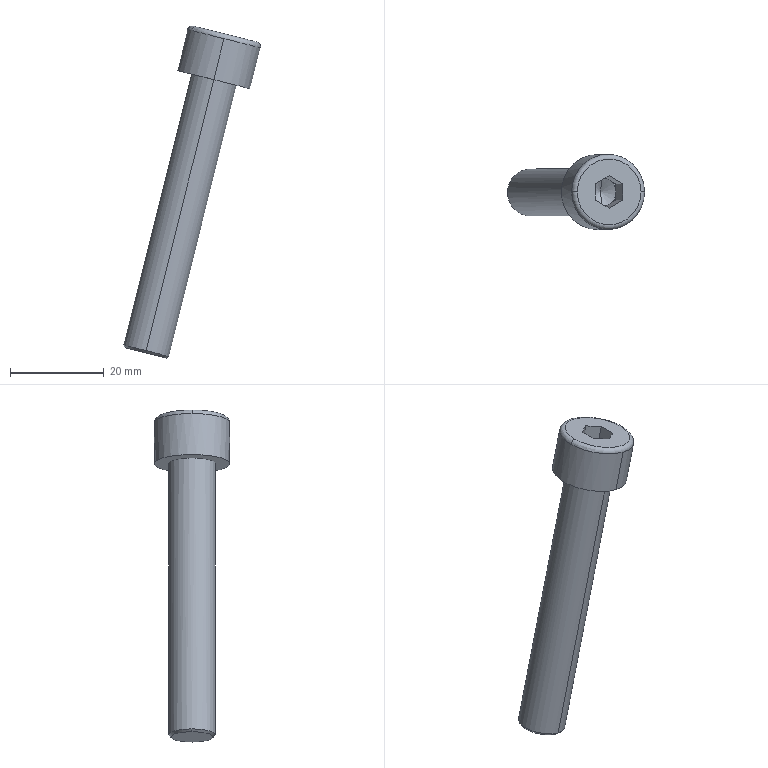Part | SolidWorks | features BaseBody 1 | 1 solid | 25 faces | box 29.213 x 16 x 70.733 mm | volume 6505 mm3 | plane 15 | cone 4 | cylinder 4 | torus 2 | commonest cylinder face diameters 10 x2 16 x2
STEP:
#1=CARTESIAN_POINT('',(-428.449,-4.,429.111));
#2=VERTEX_POINT('',#1);
#3=CARTESIAN_POINT('',(-414.865,-4.,425.724));
#4=VERTEX_POINT('',#3);
#5=CARTESIAN_POINT('',(-421.657,-4.,427.418));
#6=DIRECTION('',(0.2419,0.,0.9703));
#7=DIRECTION('',(-0.9703,0.,0.2419));
#8=AXIS2_PLACEMENT_3D('',#5,#6,#7);
#9=CIRCLE('',#8,7.);
#10=EDGE_CURVE('',#2,#4,#9,.T.);
#11=ORIENTED_EDGE('',*,*,#10,.F.);
#12=CARTESIAN_POINT('',(-429.661,-4.,428.382));
#13=VERTEX_POINT('',#12);
#14=CARTESIAN_POINT('',(-428.691,-4.,428.14));
#15=DIRECTION('',(0.,-1.,0.));
#16=DIRECTION('',(1.,0.,0.));
#17=AXIS2_PLACEMENT_3D('',#14,#15,#16);
#18=CIRCLE('',#17,1.);
#19=EDGE_CURVE('',#2,#13,#18,.T.);
#20=ORIENTED_EDGE('',*,*,#19,.T.);
#21=CARTESIAN_POINT('',(-421.899,-12.,426.447));
#22=VERTEX_POINT('',#21);
#23=CARTESIAN_POINT('',(-421.899,-4.,426.447));
#24=DIRECTION('',(-0.2419,0.,-0.9703));
#25=DIRECTION('',(-0.9703,0.,0.2419));
#26=AXIS2_PLACEMENT_3D('',#23,#24,#25);
#27=CIRCLE('',#26,8.);
#28=EDGE_CURVE('',#22,#13,#27,.T.);
#29=ORIENTED_EDGE('',*,*,#28,.F.);
#30=CARTESIAN_POINT('',(-414.136,-4.,424.512));
#31=VERTEX_POINT('',#30);
#32=CARTESIAN_POINT('',(-421.899,-4.,426.447));
#33=DIRECTION('',(-0.2419,0.,-0.9703));
#34=DIRECTION('',(-0.9703,0.,0.2419));
#35=AXIS2_PLACEMENT_3D('',#32,#33,#34);
#36=CIRCLE('',#35,8.);
#37=EDGE_CURVE('',#31,#22,#36,.T.);
#38=ORIENTED_EDGE('',*,*,#37,.F.);
#39=CARTESIAN_POINT('',(-415.107,-4.,424.754));
#40=DIRECTION('',(0.,1.,0.));
#41=DIRECTION('',(0.,0.,1.));
#42=AXIS2_PLACEMENT_3D('',#39,#40,#41);
#43=CIRCLE('',#42,1.);
#44=EDGE_CURVE('',#4,#31,#43,.T.);
#45=ORIENTED_EDGE('',*,*,#44,.F.);
#46=EDGE_LOOP('',(#11,#20,#29,#38,#45));
#47=FACE_OUTER_BOUND('',#46,.T.);
#48=CARTESIAN_POINT('',(-421.899,-4.,426.447));
#49=DIRECTION('',(-0.2419,0.,-0.9703));
#50=DIRECTION('',(0.9703,0.,-0.2419));
#51=AXIS2_PLACEMENT_3D('',#48,#49,#50);
#52=TOROIDAL_SURFACE('',#51,7.,1.);
#53=ADVANCED_FACE('',(#47),#52,.T.);
#54=CARTESIAN_POINT('',(-434.222,-4.,358.408));
#55=VERTEX_POINT('',#54);
#56=CARTESIAN_POINT('',(-442.955,-4.,360.585));
#57=VERTEX_POINT('',#56);
#58=CARTESIAN_POINT('',(-438.589,-4.,359.496));
#59=DIRECTION('',(-0.2419,0.,-0.9703));
#60=DIRECTION('',(-0.9703,0.,0.2419));
#61=AXIS2_PLACEMENT_3D('',#58,#59,#60);
#62=CIRCLE('',#61,4.5);
#63=EDGE_CURVE('',#55,#57,#62,.T.);
#64=ORIENTED_EDGE('',*,*,#63,.F.);
#65=CARTESIAN_POINT('',(-433.616,-4.,358.772));
#66=VERTEX_POINT('',#65);
#67=CARTESIAN_POINT('',(-434.222,-4.,358.408));
#68=DIRECTION('',(0.8571,0.,0.5151));
#69=VECTOR('',#68,1000.);
#70=LINE('',#67,#69);
#71=EDGE_CURVE('',#55,#66,#70,.T.);
#72=ORIENTED_EDGE('',*,*,#71,.T.);
#73=CARTESIAN_POINT('',(-438.468,-9.,359.981));
#74=VERTEX_POINT('',#73);
#75=CARTESIAN_POINT('',(-438.468,-4.,359.981));
#76=DIRECTION('',(0.2419,0.,0.9703));
#77=DIRECTION('',(0.9703,0.,-0.2419));
#78=AXIS2_PLACEMENT_3D('',#75,#76,#77);
#79=CIRCLE('',#78,5.);
#80=EDGE_CURVE('',#74,#66,#79,.T.);
#81=ORIENTED_EDGE('',*,*,#80,.F.);
#82=CARTESIAN_POINT('',(-443.319,-4.,361.191));
#83=VERTEX_POINT('',#82);
#84=CARTESIAN_POINT('',(-438.468,-4.,359.981));
#85=DIRECTION('',(0.2419,0.,0.9703));
#86=DIRECTION('',(0.9703,0.,-0.2419));
#87=AXIS2_PLACEMENT_3D('',#84,#85,#86);
#88=CIRCLE('',#87,5.);
#89=EDGE_CURVE('',#83,#74,#88,.T.);
#90=ORIENTED_EDGE('',*,*,#89,.F.);
#91=CARTESIAN_POINT('',(-442.955,-4.,360.585));
#92=DIRECTION('',(-0.5151,0.,0.8571));
#93=VECTOR('',#92,1000.);
#94=LINE('',#91,#93);
#95=EDGE_CURVE('',#57,#83,#94,.T.);
#96=ORIENTED_EDGE('',*,*,#95,.F.);
#97=EDGE_LOOP('',(#64,#72,#81,#90,#96));
#98=FACE_OUTER_BOUND('',#97,.T.);
#99=CARTESIAN_POINT('',(-438.589,-4.,359.496));
#100=DIRECTION('',(0.2419,0.,0.9703));
#101=DIRECTION('',(-0.9703,0.,0.2419));
#102=AXIS2_PLACEMENT_3D('',#99,#100,#101);
#103=CONICAL_SURFACE('',#102,4.5,0.7854);
#104=ADVANCED_FACE('',(#98),#103,.T.);
#105=CARTESIAN_POINT('',(-423.527,-4.,419.915));
#106=VERTEX_POINT('',#105);
#107=CARTESIAN_POINT('',(-423.108,-1.,421.596));
#108=VERTEX_POINT('',#107);
#109=CARTESIAN_POINT('',(-423.311,-2.451,420.783));
#110=DIRECTION('',(0.1209,0.866,0.4852));
#111=VECTOR('',#110,1000.);
#112=LINE('',#109,#111);
#113=EDGE_CURVE('',#106,#108,#112,.T.);
#114=ORIENTED_EDGE('',*,*,#113,.F.);
#115=CARTESIAN_POINT('',(-423.108,-7.,421.596));
#116=VERTEX_POINT('',#115);
#117=CARTESIAN_POINT('',(-423.311,-5.549,420.783));
#118=DIRECTION('',(0.1209,-0.866,0.4852));
#119=VECTOR('',#118,1000.);
#120=LINE('',#117,#119);
#121=EDGE_CURVE('',#106,#116,#120,.T.);
#122=ORIENTED_EDGE('',*,*,#121,.T.);
#123=CARTESIAN_POINT('',(-421.653,-6.598,421.233));
#124=VERTEX_POINT('',#123);
#125=CARTESIAN_POINT('',(-423.108,-4.,421.596));
#126=DIRECTION('',(-0.2419,0.,-0.9703));
#127=DIRECTION('',(0.,-1.,0.));
#128=AXIS2_PLACEMENT_3D('',#125,#126,#127);
#129=CIRCLE('',#128,3.);
#130=EDGE_CURVE('',#124,#116,#129,.T.);
#131=ORIENTED_EDGE('',*,*,#130,.F.);
#132=CARTESIAN_POINT('',(-420.197,-4.,420.87));
#133=VERTEX_POINT('',#132);
#134=CARTESIAN_POINT('',(-423.108,-4.,421.596));
#135=DIRECTION('',(-0.2419,0.,-0.9703));
#136=DIRECTION('',(0.9703,0.,-0.2419));
#137=AXIS2_PLACEMENT_3D('',#134,#135,#136);
#138=CIRCLE('',#137,3.);
#139=EDGE_CURVE('',#133,#124,#138,.T.);
#140=ORIENTED_EDGE('',*,*,#139,.F.);
#141=CARTESIAN_POINT('',(-421.653,-1.402,421.233));
#142=VERTEX_POINT('',#141);
#143=CARTESIAN_POINT('',(-423.108,-4.,421.596));
#144=DIRECTION('',(-0.2419,0.,-0.9703));
#145=DIRECTION('',(0.4852,0.866,-0.1209));
#146=AXIS2_PLACEMENT_3D('',#143,#144,#145);
#147=CIRCLE('',#146,3.);
#148=EDGE_CURVE('',#142,#133,#147,.T.);
#149=ORIENTED_EDGE('',*,*,#148,.F.);
#150=CARTESIAN_POINT('',(-423.108,-4.,421.596));
#151=DIRECTION('',(-0.2419,0.,-0.9703));
#152=DIRECTION('',(-0.4852,0.866,0.1209));
#153=AXIS2_PLACEMENT_3D('',#150,#151,#152);
#154=CIRCLE('',#153,3.);
#155=EDGE_CURVE('',#108,#142,#154,.T.);
#156=ORIENTED_EDGE('',*,*,#155,.F.);
#157=EDGE_LOOP('',(#114,#122,#131,#140,#149,#156));
#158=FACE_OUTER_BOUND('',#157,.T.);
#159=CARTESIAN_POINT('',(-423.311,-4.,420.783));
#160=DIRECTION('',(0.2419,0.,0.9703));
#161=DIRECTION('',(0.,1.,0.));
#162=AXIS2_PLACEMENT_3D('',#159,#160,#161);
#163=CONICAL_SURFACE('',#162,1.549,1.047);
#164=ADVANCED_FACE('',(#158),#163,.F.);
#165=CARTESIAN_POINT('',(-424.076,-12.,417.715));
#166=VERTEX_POINT('',#165);
#167=CARTESIAN_POINT('',(-424.076,4.,417.715));
#168=VERTEX_POINT('',#167);
#169=CARTESIAN_POINT('',(-424.076,-4.,417.715));
#170=DIRECTION('',(-0.2419,0.,-0.9703));
#171=DIRECTION('',(-0.9703,0.,0.2419));
#172=AXIS2_PLACEMENT_3D('',#169,#170,#171);
#173=CIRCLE('',#172,8.);
#174=EDGE_CURVE('',#166,#168,#173,.T.);
#175=ORIENTED_EDGE('',*,*,#174,.F.);
#176=CARTESIAN_POINT('',(-424.076,-12.,417.715));
#177=DIRECTION('',(0.2419,0.,0.9703));
#178=VECTOR('',#177,1000.);
#179=LINE('',#176,#178);
#180=EDGE_CURVE('',#166,#22,#179,.T.);
#181=ORIENTED_EDGE('',*,*,#180,.T.);
#182=ORIENTED_EDGE('',*,*,#28,.T.);
#183=CARTESIAN_POINT('',(-421.899,4.,426.447));
#184=VERTEX_POINT('',#183);
#185=CARTESIAN_POINT('',(-421.899,-4.,426.447));
#186=DIRECTION('',(-0.2419,0.,-0.9703));
#187=DIRECTION('',(-0.9703,0.,0.2419));
#188=AXIS2_PLACEMENT_3D('',#185,#186,#187);
#189=CIRCLE('',#188,8.);
#190=EDGE_CURVE('',#13,#184,#189,.T.);
#191=ORIENTED_EDGE('',*,*,#190,.T.);
#192=CARTESIAN_POINT('',(-424.076,4.,417.715));
#193=DIRECTION('',(0.2419,0.,0.9703));
#194=VECTOR('',#193,1000.);
#195=LINE('',#192,#194);
#196=EDGE_CURVE('',#168,#184,#195,.T.);
#197=ORIENTED_EDGE('',*,*,#196,.F.);
#198=EDGE_LOOP('',(#175,#181,#182,#191,#197));
#199=FACE_OUTER_BOUND('',#198,.T.);
#200=CARTESIAN_POINT('',(-424.076,-4.,417.715));
#201=DIRECTION('',(0.2419,0.,0.9703));
#202=DIRECTION('',(0.,1.,0.));
#203=AXIS2_PLACEMENT_3D('',#200,#201,#202);
#204=CYLINDRICAL_SURFACE('',#203,8.);
#205=ADVANCED_FACE('',(#199),#204,.T.);
#206=CARTESIAN_POINT('',(-438.468,1.,359.981));
#207=VERTEX_POINT('',#206);
#208=CARTESIAN_POINT('',(-438.468,-4.,359.981));
#209=DIRECTION('',(0.2419,0.,0.9703));
#210=DIRECTION('',(0.9703,0.,-0.2419));
#211=AXIS2_PLACEMENT_3D('',#208,#209,#210);
#212=CIRCLE('',#211,5.);
#213=EDGE_CURVE('',#207,#83,#212,.T.);
#214=ORIENTED_EDGE('',*,*,#213,.T.);
#215=ORIENTED_EDGE('',*,*,#89,.T.);
#216=CARTESIAN_POINT('',(-424.076,-9.,417.715));
#217=VERTEX_POINT('',#216);
#218=CARTESIAN_POINT('',(-426.494,-9.,408.012));
#219=DIRECTION('',(0.2419,0.,0.9703));
#220=VECTOR('',#219,1000.);
#221=LINE('',#218,#220);
#222=EDGE_CURVE('',#74,#217,#221,.T.);
#223=ORIENTED_EDGE('',*,*,#222,.T.);
#224=CARTESIAN_POINT('',(-424.076,1.,417.715));
#225=VERTEX_POINT('',#224);
#226=CARTESIAN_POINT('',(-424.076,-4.,417.715));
#227=DIRECTION('',(-0.2419,0.,-0.9703));
#228=DIRECTION('',(-0.9703,0.,0.2419));
#229=AXIS2_PLACEMENT_3D('',#226,#227,#228);
#230=CIRCLE('',#229,5.);
#231=EDGE_CURVE('',#217,#225,#230,.T.);
#232=ORIENTED_EDGE('',*,*,#231,.T.);
#233=CARTESIAN_POINT('',(-426.494,1.,408.012));
#234=DIRECTION('',(0.2419,0.,0.9703));
#235=VECTOR('',#234,1000.);
#236=LINE('',#233,#235);
#237=EDGE_CURVE('',#207,#225,#236,.T.);
#238=ORIENTED_EDGE('',*,*,#237,.F.);
#239=EDGE_LOOP('',(#214,#215,#223,#232,#238));
#240=FACE_OUTER_BOUND('',#239,.T.);
#241=CARTESIAN_POINT('',(-426.494,-4.,408.012));
#242=DIRECTION('',(0.2419,0.,0.9703));
#243=DIRECTION('',(0.,1.,0.));
#244=AXIS2_PLACEMENT_3D('',#241,#242,#243);
#245=CYLINDRICAL_SURFACE('',#244,5.);
#246=ADVANCED_FACE('',(#240),#245,.T.);
#247=CARTESIAN_POINT('',(-438.589,-4.,359.496));
#248=DIRECTION('',(-0.2419,0.,-0.9703));
#249=DIRECTION('',(-0.9703,0.,0.2419));
#250=AXIS2_PLACEMENT_3D('',#247,#248,#249);
#251=CIRCLE('',#250,4.5);
#252=EDGE_CURVE('',#57,#55,#251,.T.);
#253=ORIENTED_EDGE('',*,*,#252,.T.);
#254=ORIENTED_EDGE('',*,*,#63,.T.);
#255=EDGE_LOOP('',(#253,#254));
#256=FACE_OUTER_BOUND('',#255,.T.);
#257=CARTESIAN_POINT('',(-438.589,-4.,359.496));
#258=DIRECTION('',(-0.2419,0.,-0.9703));
#259=DIRECTION('',(-0.9703,0.,0.2419));
#260=AXIS2_PLACEMENT_3D('',#257,#258,#259);
#261=PLANE('',#260);
#262=ADVANCED_FACE('',(#256),#261,.T.);
#263=ORIENTED_EDGE('',*,*,#222,.F.);
#264=ORIENTED_EDGE('',*,*,#80,.T.);
#265=CARTESIAN_POINT('',(-438.468,-4.,359.981));
#266=DIRECTION('',(0.2419,0.,0.9703));
#267=DIRECTION('',(0.9703,0.,-0.2419));
#268=AXIS2_PLACEMENT_3D('',#265,#266,#267);
#269=CIRCLE('',#268,5.);
#270=EDGE_CURVE('',#66,#207,#269,.T.);
#271=ORIENTED_EDGE('',*,*,#270,.T.);
#272=ORIENTED_EDGE('',*,*,#237,.T.);
#273=CARTESIAN_POINT('',(-424.076,-4.,417.715));
#274=DIRECTION('',(-0.2419,0.,-0.9703));
#275=DIRECTION('',(-0.9703,0.,0.2419));
#276=AXIS2_PLACEMENT_3D('',#273,#274,#275);
#277=CIRCLE('',#276,5.);
#278=EDGE_CURVE('',#225,#217,#277,.T.);
#279=ORIENTED_EDGE('',*,*,#278,.T.);
#280=EDGE_LOOP('',(#263,#264,#271,#272,#279));
#281=FACE_OUTER_BOUND('',#280,.T.);
#282=CARTESIAN_POINT('',(-426.494,-4.,408.012));
#283=DIRECTION('',(0.2419,0.,0.9703));
#284=DIRECTION('',(0.,1.,0.));
#285=AXIS2_PLACEMENT_3D('',#282,#283,#284);
#286=CYLINDRICAL_SURFACE('',#285,5.);
#287=ADVANCED_FACE('',(#281),#286,.T.);
#288=ORIENTED_EDGE('',*,*,#278,.F.);
#289=ORIENTED_EDGE('',*,*,#231,.F.);
#290=EDGE_LOOP('',(#288,#289));
#291=FACE_BOUND('',#290,.T.);
#292=CARTESIAN_POINT('',(-424.076,-4.,417.715));
#293=DIRECTION('',(-0.2419,0.,-0.9703));
#294=DIRECTION('',(-0.9703,0.,0.2419));
#295=AXIS2_PLACEMENT_3D('',#292,#293,#294);
#296=CIRCLE('',#295,8.);
#297=EDGE_CURVE('',#168,#166,#296,.T.);
#298=ORIENTED_EDGE('',*,*,#297,.T.);
#299=ORIENTED_EDGE('',*,*,#174,.T.);
#300=EDGE_LOOP('',(#298,#299));
#301=FACE_OUTER_BOUND('',#300,.T.);
#302=CARTESIAN_POINT('',(-424.076,-4.,417.715));
#303=DIRECTION('',(-0.2419,0.,-0.9703));
#304=DIRECTION('',(-0.9703,0.,0.2419));
#305=AXIS2_PLACEMENT_3D('',#302,#303,#304);
#306=PLANE('',#305);
#307=ADVANCED_FACE('',(#291,#301),#306,.T.);
#308=ORIENTED_EDGE('',*,*,#180,.F.);
#309=ORIENTED_EDGE('',*,*,#297,.F.);
#310=ORIENTED_EDGE('',*,*,#196,.T.);
#311=CARTESIAN_POINT('',(-421.899,-4.,426.447));
#312=DIRECTION('',(-0.2419,0.,-0.9703));
#313=DIRECTION('',(-0.9703,0.,0.2419));
#314=AXIS2_PLACEMENT_3D('',#311,#312,#313);
#315=CIRCLE('',#314,8.);
#316=EDGE_CURVE('',#184,#31,#315,.T.);
#317=ORIENTED_EDGE('',*,*,#316,.T.);
#318=ORIENTED_EDGE('',*,*,#37,.T.);
#319=EDGE_LOOP('',(#308,#309,#310,#317,#318));
#320=FACE_OUTER_BOUND('',#319,.T.);
#321=CARTESIAN_POINT('',(-424.076,-4.,417.715));
#322=DIRECTION('',(0.2419,0.,0.9703));
#323=DIRECTION('',(0.,1.,0.));
#324=AXIS2_PLACEMENT_3D('',#321,#322,#323);
#325=CYLINDRICAL_SURFACE('',#324,8.);
#326=ADVANCED_FACE('',(#320),#325,.T.);
#327=CARTESIAN_POINT('',(-418.746,-2.268,426.692));
#328=VERTEX_POINT('',#327);
#329=CARTESIAN_POINT('',(-418.746,-5.732,426.692));
#330=VERTEX_POINT('',#329);
#331=CARTESIAN_POINT('',(-418.746,-2.268,426.692));
#332=DIRECTION('',(0.,-1.,0.));
#333=VECTOR('',#332,1000.);
#334=LINE('',#331,#333);
#335=EDGE_CURVE('',#328,#330,#334,.T.);
#336=ORIENTED_EDGE('',*,*,#335,.T.);
#337=CARTESIAN_POINT('',(-421.657,-7.464,427.418));
#338=VERTEX_POINT('',#337);
#339=CARTESIAN_POINT('',(-418.746,-5.732,426.692));
#340=DIRECTION('',(-0.8403,-0.5,0.2095));
#341=VECTOR('',#340,1000.);
#342=LINE('',#339,#341);
#343=EDGE_CURVE('',#330,#338,#342,.T.);
#344=ORIENTED_EDGE('',*,*,#343,.T.);
#345=CARTESIAN_POINT('',(-424.568,-5.732,428.143));
#346=VERTEX_POINT('',#345);
#347=CARTESIAN_POINT('',(-421.657,-7.464,427.418));
#348=DIRECTION('',(-0.8403,0.5,0.2095));
#349=VECTOR('',#348,1000.);
#350=LINE('',#347,#349);
#351=EDGE_CURVE('',#338,#346,#350,.T.);
#352=ORIENTED_EDGE('',*,*,#351,.T.);
#353=CARTESIAN_POINT('',(-424.568,-2.268,428.143));
#354=VERTEX_POINT('',#353);
#355=CARTESIAN_POINT('',(-424.568,-5.732,428.143));
#356=DIRECTION('',(0.,1.,0.));
#357=VECTOR('',#356,1000.);
#358=LINE('',#355,#357);
#359=EDGE_CURVE('',#346,#354,#358,.T.);
#360=ORIENTED_EDGE('',*,*,#359,.T.);
#361=CARTESIAN_POINT('',(-421.657,-0.5359,427.418));
#362=VERTEX_POINT('',#361);
#363=CARTESIAN_POINT('',(-424.568,-2.268,428.143));
#364=DIRECTION('',(0.8403,0.5,-0.2095));
#365=VECTOR('',#364,1000.);
#366=LINE('',#363,#365);
#367=EDGE_CURVE('',#354,#362,#366,.T.);
#368=ORIENTED_EDGE('',*,*,#367,.T.);
#369=CARTESIAN_POINT('',(-421.657,-0.5359,427.418));
#370=DIRECTION('',(0.8403,-0.5,-0.2095));
#371=VECTOR('',#370,1000.);
#372=LINE('',#369,#371);
#373=EDGE_CURVE('',#362,#328,#372,.T.);
#374=ORIENTED_EDGE('',*,*,#373,.T.);
#375=EDGE_LOOP('',(#336,#344,#352,#360,#368,#374));
#376=FACE_BOUND('',#375,.T.);
#377=CARTESIAN_POINT('',(-421.657,-4.,427.418));
#378=DIRECTION('',(0.2419,0.,0.9703));
#379=DIRECTION('',(-0.9703,0.,0.2419));
#380=AXIS2_PLACEMENT_3D('',#377,#378,#379);
#381=CIRCLE('',#380,7.);
#382=EDGE_CURVE('',#4,#2,#381,.T.);
#383=ORIENTED_EDGE('',*,*,#382,.T.);
#384=ORIENTED_EDGE('',*,*,#10,.T.);
#385=EDGE_LOOP('',(#383,#384));
#386=FACE_OUTER_BOUND('',#385,.T.);
#387=CARTESIAN_POINT('',(-421.657,-4.,427.418));
#388=DIRECTION('',(-0.2419,0.,-0.9703));
#389=DIRECTION('',(-0.9703,0.,0.2419));
#390=AXIS2_PLACEMENT_3D('',#387,#388,#389);
#391=PLANE('',#390);
#392=ADVANCED_FACE('',(#376,#386),#391,.F.);
#393=CARTESIAN_POINT('',(-420.197,-5.732,420.87));
#394=VERTEX_POINT('',#393);
#395=CARTESIAN_POINT('',(-419.23,-5.732,424.751));
#396=DIRECTION('',(-0.2419,0.,-0.9703));
#397=VECTOR('',#396,1000.);
#398=LINE('',#395,#397);
#399=EDGE_CURVE('',#330,#394,#398,.T.);
#400=ORIENTED_EDGE('',*,*,#399,.F.);
#401=ORIENTED_EDGE('',*,*,#335,.F.);
#402=CARTESIAN_POINT('',(-420.197,-2.268,420.87));
#403=VERTEX_POINT('',#402);
#404=CARTESIAN_POINT('',(-419.23,-2.268,424.751));
#405=DIRECTION('',(-0.2419,0.,-0.9703));
#406=VECTOR('',#405,1000.);
#407=LINE('',#404,#406);
#408=EDGE_CURVE('',#328,#403,#407,.T.);
#409=ORIENTED_EDGE('',*,*,#408,.T.);
#410=CARTESIAN_POINT('',(-420.197,-4.,420.87));
#411=DIRECTION('',(0.,1.,0.));
#412=VECTOR('',#411,1000.);
#413=LINE('',#410,#412);
#414=EDGE_CURVE('',#133,#403,#413,.T.);
#415=ORIENTED_EDGE('',*,*,#414,.F.);
#416=CARTESIAN_POINT('',(-420.197,-5.732,420.87));
#417=DIRECTION('',(0.,1.,0.));
#418=VECTOR('',#417,1000.);
#419=LINE('',#416,#418);
#420=EDGE_CURVE('',#394,#133,#419,.T.);
#421=ORIENTED_EDGE('',*,*,#420,.F.);
#422=EDGE_LOOP('',(#400,#401,#409,#415,#421));
#423=FACE_OUTER_BOUND('',#422,.T.);
#424=CARTESIAN_POINT('',(-420.197,-2.268,420.87));
#425=DIRECTION('',(-0.9703,0.,0.2419));
#426=DIRECTION('',(0.,1.,0.));
#427=AXIS2_PLACEMENT_3D('',#424,#425,#426);
#428=PLANE('',#427);
#429=ADVANCED_FACE('',(#423),#428,.T.);
#430=CARTESIAN_POINT('',(-423.108,-7.464,421.596));
#431=VERTEX_POINT('',#430);
#432=CARTESIAN_POINT('',(-422.141,-7.464,425.477));
#433=DIRECTION('',(-0.2419,0.,-0.9703));
#434=VECTOR('',#433,1000.);
#435=LINE('',#432,#434);
#436=EDGE_CURVE('',#338,#431,#435,.T.);
#437=ORIENTED_EDGE('',*,*,#436,.F.);
#438=ORIENTED_EDGE('',*,*,#343,.F.);
#439=ORIENTED_EDGE('',*,*,#399,.T.);
#440=CARTESIAN_POINT('',(-421.653,-6.598,421.233));
#441=DIRECTION('',(0.8403,0.5,-0.2095));
#442=VECTOR('',#441,1000.);
#443=LINE('',#440,#442);
#444=EDGE_CURVE('',#124,#394,#443,.T.);
#445=ORIENTED_EDGE('',*,*,#444,.F.);
#446=CARTESIAN_POINT('',(-423.108,-7.464,421.596));
#447=DIRECTION('',(0.8403,0.5,-0.2095));
#448=VECTOR('',#447,1000.);
#449=LINE('',#446,#448);
#450=EDGE_CURVE('',#431,#124,#449,.T.);
#451=ORIENTED_EDGE('',*,*,#450,.F.);
#452=EDGE_LOOP('',(#437,#438,#439,#445,#451));
#453=FACE_OUTER_BOUND('',#452,.T.);
#454=CARTESIAN_POINT('',(-420.197,-5.732,420.87));
#455=DIRECTION('',(-0.4852,0.866,0.1209));
#456=DIRECTION('',(0.2419,0.,0.9703));
#457=AXIS2_PLACEMENT_3D('',#454,#455,#456);
#458=PLANE('',#457);
#459=ADVANCED_FACE('',(#453),#458,.T.);
#460=CARTESIAN_POINT('',(-426.019,-5.732,422.321));
#461=VERTEX_POINT('',#460);
#462=CARTESIAN_POINT('',(-425.051,-5.732,426.203));
#463=DIRECTION('',(-0.2419,0.,-0.9703));
#464=VECTOR('',#463,1000.);
#465=LINE('',#462,#464);
#466=EDGE_CURVE('',#346,#461,#465,.T.);
#467=ORIENTED_EDGE('',*,*,#466,.F.);
#468=ORIENTED_EDGE('',*,*,#351,.F.);
#469=ORIENTED_EDGE('',*,*,#436,.T.);
#470=CARTESIAN_POINT('',(-424.564,-6.598,421.959));
#471=VERTEX_POINT('',#470);
#472=CARTESIAN_POINT('',(-424.564,-6.598,421.959));
#473=DIRECTION('',(0.8403,-0.5,-0.2095));
#474=VECTOR('',#473,1000.);
#475=LINE('',#472,#474);
#476=EDGE_CURVE('',#471,#431,#475,.T.);
#477=ORIENTED_EDGE('',*,*,#476,.F.);
#478=CARTESIAN_POINT('',(-426.019,-5.732,422.321));
#479=DIRECTION('',(0.8403,-0.5,-0.2095));
#480=VECTOR('',#479,1000.);
#481=LINE('',#478,#480);
#482=EDGE_CURVE('',#461,#471,#481,.T.);
#483=ORIENTED_EDGE('',*,*,#482,.F.);
#484=EDGE_LOOP('',(#467,#468,#469,#477,#483));
#485=FACE_OUTER_BOUND('',#484,.T.);
#486=CARTESIAN_POINT('',(-423.108,-7.464,421.596));
#487=DIRECTION('',(0.4852,0.866,-0.1209));
#488=DIRECTION('',(-0.2419,0.,-0.9703));
#489=AXIS2_PLACEMENT_3D('',#486,#487,#488);
#490=PLANE('',#489);
#491=ADVANCED_FACE('',(#485),#490,.T.);
#492=CARTESIAN_POINT('',(-426.019,-2.268,422.321));
#493=VERTEX_POINT('',#492);
#494=CARTESIAN_POINT('',(-426.019,-2.268,422.321));
#495=DIRECTION('',(0.2419,0.,0.9703));
#496=VECTOR('',#495,1000.);
#497=LINE('',#494,#496);
#498=EDGE_CURVE('',#493,#354,#497,.T.);
#499=ORIENTED_EDGE('',*,*,#498,.T.);
#500=ORIENTED_EDGE('',*,*,#359,.F.);
#501=ORIENTED_EDGE('',*,*,#466,.T.);
#502=CARTESIAN_POINT('',(-426.019,-4.,422.321));
#503=VERTEX_POINT('',#502);
#504=CARTESIAN_POINT('',(-426.019,-4.,422.321));
#505=DIRECTION('',(0.,-1.,0.));
#506=VECTOR('',#505,1000.);
#507=LINE('',#504,#506);
#508=EDGE_CURVE('',#503,#461,#507,.T.);
#509=ORIENTED_EDGE('',*,*,#508,.F.);
#510=CARTESIAN_POINT('',(-426.019,-2.268,422.321));
#511=DIRECTION('',(0.,-1.,0.));
#512=VECTOR('',#511,1000.);
#513=LINE('',#510,#512);
#514=EDGE_CURVE('',#493,#503,#513,.T.);
#515=ORIENTED_EDGE('',*,*,#514,.F.);
#516=EDGE_LOOP('',(#499,#500,#501,#509,#515));
#517=FACE_OUTER_BOUND('',#516,.T.);
#518=CARTESIAN_POINT('',(-426.019,-5.732,422.321));
#519=DIRECTION('',(0.9703,0.,-0.2419));
#520=DIRECTION('',(0.,-1.,0.));
#521=AXIS2_PLACEMENT_3D('',#518,#519,#520);
#522=PLANE('',#521);
#523=ADVANCED_FACE('',(#517),#522,.T.);
#524=CARTESIAN_POINT('',(-423.108,-0.5359,421.596));
#525=VERTEX_POINT('',#524);
#526=CARTESIAN_POINT('',(-422.141,-0.5359,425.477));
#527=DIRECTION('',(-0.2419,0.,-0.9703));
#528=VECTOR('',#527,1000.);
#529=LINE('',#526,#528);
#530=EDGE_CURVE('',#362,#525,#529,.T.);
#531=ORIENTED_EDGE('',*,*,#530,.F.);
#532=ORIENTED_EDGE('',*,*,#367,.F.);
#533=ORIENTED_EDGE('',*,*,#498,.F.);
#534=CARTESIAN_POINT('',(-424.564,-1.402,421.959));
#535=VERTEX_POINT('',#534);
#536=CARTESIAN_POINT('',(-424.564,-1.402,421.959));
#537=DIRECTION('',(-0.8403,-0.5,0.2095));
#538=VECTOR('',#537,1000.);
#539=LINE('',#536,#538);
#540=EDGE_CURVE('',#535,#493,#539,.T.);
#541=ORIENTED_EDGE('',*,*,#540,.F.);
#542=CARTESIAN_POINT('',(-423.108,-0.5359,421.596));
#543=DIRECTION('',(-0.8403,-0.5,0.2095));
#544=VECTOR('',#543,1000.);
#545=LINE('',#542,#544);
#546=EDGE_CURVE('',#525,#535,#545,.T.);
#547=ORIENTED_EDGE('',*,*,#546,.F.);
#548=EDGE_LOOP('',(#531,#532,#533,#541,#547));
#549=FACE_OUTER_BOUND('',#548,.T.);
#550=CARTESIAN_POINT('',(-426.019,-2.268,422.321));
#551=DIRECTION('',(0.4852,-0.866,-0.1209));
#552=DIRECTION('',(0.,0.1383,-0.9904));
#553=AXIS2_PLACEMENT_3D('',#550,#551,#552);
#554=PLANE('',#553);
#555=ADVANCED_FACE('',(#549),#554,.T.);
#556=ORIENTED_EDGE('',*,*,#408,.F.);
#557=ORIENTED_EDGE('',*,*,#373,.F.);
#558=ORIENTED_EDGE('',*,*,#530,.T.);
#559=CARTESIAN_POINT('',(-421.653,-1.402,421.233));
#560=DIRECTION('',(-0.8403,0.5,0.2095));
#561=VECTOR('',#560,1000.);
#562=LINE('',#559,#561);
#563=EDGE_CURVE('',#142,#525,#562,.T.);
#564=ORIENTED_EDGE('',*,*,#563,.F.);
#565=CARTESIAN_POINT('',(-420.197,-2.268,420.87));
#566=DIRECTION('',(-0.8403,0.5,0.2095));
#567=VECTOR('',#566,1000.);
#568=LINE('',#565,#567);
#569=EDGE_CURVE('',#403,#142,#568,.T.);
#570=ORIENTED_EDGE('',*,*,#569,.F.);
#571=EDGE_LOOP('',(#556,#557,#558,#564,#570));
#572=FACE_OUTER_BOUND('',#571,.T.);
#573=CARTESIAN_POINT('',(-423.108,-0.5359,421.596));
#574=DIRECTION('',(-0.4852,-0.866,0.1209));
#575=DIRECTION('',(-0.8724,0.4887,0.));
#576=AXIS2_PLACEMENT_3D('',#573,#574,#575);
#577=PLANE('',#576);
#578=ADVANCED_FACE('',(#572),#577,.T.);
#579=ORIENTED_EDGE('',*,*,#569,.T.);
#580=ORIENTED_EDGE('',*,*,#148,.T.);
#581=ORIENTED_EDGE('',*,*,#414,.T.);
#582=EDGE_LOOP('',(#579,#580,#581));
#583=FACE_OUTER_BOUND('',#582,.T.);
#584=CARTESIAN_POINT('',(-423.108,-0.5359,421.596));
#585=DIRECTION('',(-0.2419,0.,-0.9703));
#586=DIRECTION('',(-0.9703,0.,0.2419));
#587=AXIS2_PLACEMENT_3D('',#584,#585,#586);
#588=PLANE('',#587);
#589=ADVANCED_FACE('',(#583),#588,.F.);
#590=ORIENTED_EDGE('',*,*,#420,.T.);
#591=ORIENTED_EDGE('',*,*,#139,.T.);
#592=ORIENTED_EDGE('',*,*,#444,.T.);
#593=EDGE_LOOP('',(#590,#591,#592));
#594=FACE_OUTER_BOUND('',#593,.T.);
#595=CARTESIAN_POINT('',(-423.108,-0.5359,421.596));
#596=DIRECTION('',(-0.2419,0.,-0.9703));
#597=DIRECTION('',(-0.9703,0.,0.2419));
#598=AXIS2_PLACEMENT_3D('',#595,#596,#597);
#599=PLANE('',#598);
#600=ADVANCED_FACE('',(#594),#599,.F.);
#601=ORIENTED_EDGE('',*,*,#450,.T.);
#602=ORIENTED_EDGE('',*,*,#130,.T.);
#603=CARTESIAN_POINT('',(-423.108,-4.,421.596));
#604=DIRECTION('',(-0.2419,0.,-0.9703));
#605=DIRECTION('',(0.,-1.,0.));
#606=AXIS2_PLACEMENT_3D('',#603,#604,#605);
#607=CIRCLE('',#606,3.);
#608=EDGE_CURVE('',#116,#471,#607,.T.);
#609=ORIENTED_EDGE('',*,*,#608,.T.);
#610=ORIENTED_EDGE('',*,*,#476,.T.);
#611=EDGE_LOOP('',(#601,#602,#609,#610));
#612=FACE_OUTER_BOUND('',#611,.T.);
#613=CARTESIAN_POINT('',(-423.108,-0.5359,421.596));
#614=DIRECTION('',(-0.2419,0.,-0.9703));
#615=DIRECTION('',(-0.9703,0.,0.2419));
#616=AXIS2_PLACEMENT_3D('',#613,#614,#615);
#617=PLANE('',#616);
#618=ADVANCED_FACE('',(#612),#617,.F.);
#619=ORIENTED_EDGE('',*,*,#482,.T.);
#620=CARTESIAN_POINT('',(-423.108,-4.,421.596));
#621=DIRECTION('',(-0.2419,0.,-0.9703));
#622=DIRECTION('',(-0.4852,-0.866,0.1209));
#623=AXIS2_PLACEMENT_3D('',#620,#621,#622);
#624=CIRCLE('',#623,3.);
#625=EDGE_CURVE('',#471,#503,#624,.T.);
#626=ORIENTED_EDGE('',*,*,#625,.T.);
#627=ORIENTED_EDGE('',*,*,#508,.T.);
#628=EDGE_LOOP('',(#619,#626,#627));
#629=FACE_OUTER_BOUND('',#628,.T.);
#630=CARTESIAN_POINT('',(-423.108,-0.5359,421.596));
#631=DIRECTION('',(-0.2419,0.,-0.9703));
#632=DIRECTION('',(-0.9703,0.,0.2419));
#633=AXIS2_PLACEMENT_3D('',#630,#631,#632);
#634=PLANE('',#633);
#635=ADVANCED_FACE('',(#629),#634,.F.);
#636=ORIENTED_EDGE('',*,*,#514,.T.);
#637=CARTESIAN_POINT('',(-423.108,-4.,421.596));
#638=DIRECTION('',(-0.2419,0.,-0.9703));
#639=DIRECTION('',(-0.9703,0.,0.2419));
#640=AXIS2_PLACEMENT_3D('',#637,#638,#639);
#641=CIRCLE('',#640,3.);
#642=EDGE_CURVE('',#503,#535,#641,.T.);
#643=ORIENTED_EDGE('',*,*,#642,.T.);
#644=ORIENTED_EDGE('',*,*,#540,.T.);
#645=EDGE_LOOP('',(#636,#643,#644));
#646=FACE_OUTER_BOUND('',#645,.T.);
#647=CARTESIAN_POINT('',(-423.108,-0.5359,421.596));
#648=DIRECTION('',(-0.2419,0.,-0.9703));
#649=DIRECTION('',(-0.9703,0.,0.2419));
#650=AXIS2_PLACEMENT_3D('',#647,#648,#649);
#651=PLANE('',#650);
#652=ADVANCED_FACE('',(#646),#651,.F.);
#653=ORIENTED_EDGE('',*,*,#546,.T.);
#654=CARTESIAN_POINT('',(-423.108,-4.,421.596));
#655=DIRECTION('',(-0.2419,0.,-0.9703));
#656=DIRECTION('',(-0.4852,0.866,0.1209));
#657=AXIS2_PLACEMENT_3D('',#654,#655,#656);
#658=CIRCLE('',#657,3.);
#659=EDGE_CURVE('',#535,#108,#658,.T.);
#660=ORIENTED_EDGE('',*,*,#659,.T.);
#661=ORIENTED_EDGE('',*,*,#155,.T.);
#662=ORIENTED_EDGE('',*,*,#563,.T.);
#663=EDGE_LOOP('',(#653,#660,#661,#662));
#664=FACE_OUTER_BOUND('',#663,.T.);
#665=CARTESIAN_POINT('',(-423.108,-0.5359,421.596));
#666=DIRECTION('',(-0.2419,0.,-0.9703));
#667=DIRECTION('',(-0.9703,0.,0.2419));
#668=AXIS2_PLACEMENT_3D('',#665,#666,#667);
#669=PLANE('',#668);
#670=ADVANCED_FACE('',(#664),#669,.F.);
#671=ORIENTED_EDGE('',*,*,#121,.F.);
#672=ORIENTED_EDGE('',*,*,#113,.T.);
#673=ORIENTED_EDGE('',*,*,#659,.F.);
#674=ORIENTED_EDGE('',*,*,#642,.F.);
#675=ORIENTED_EDGE('',*,*,#625,.F.);
#676=ORIENTED_EDGE('',*,*,#608,.F.);
#677=EDGE_LOOP('',(#671,#672,#673,#674,#675,#676));
#678=FACE_OUTER_BOUND('',#677,.T.);
#679=CARTESIAN_POINT('',(-423.311,-4.,420.783));
#680=DIRECTION('',(0.2419,0.,0.9703));
#681=DIRECTION('',(0.,1.,0.));
#682=AXIS2_PLACEMENT_3D('',#679,#680,#681);
#683=CONICAL_SURFACE('',#682,1.549,1.047);
#684=ADVANCED_FACE('',(#678),#683,.F.);
#685=ORIENTED_EDGE('',*,*,#71,.F.);
#686=ORIENTED_EDGE('',*,*,#252,.F.);
#687=ORIENTED_EDGE('',*,*,#95,.T.);
#688=ORIENTED_EDGE('',*,*,#213,.F.);
#689=ORIENTED_EDGE('',*,*,#270,.F.);
#690=EDGE_LOOP('',(#685,#686,#687,#688,#689));
#691=FACE_OUTER_BOUND('',#690,.T.);
#692=CARTESIAN_POINT('',(-438.589,-4.,359.496));
#693=DIRECTION('',(0.2419,0.,0.9703));
#694=DIRECTION('',(-0.9703,0.,0.2419));
#695=AXIS2_PLACEMENT_3D('',#692,#693,#694);
#696=CONICAL_SURFACE('',#695,4.5,0.7854);
#697=ADVANCED_FACE('',(#691),#696,.T.);
#698=ORIENTED_EDGE('',*,*,#19,.F.);
#699=ORIENTED_EDGE('',*,*,#382,.F.);
#700=ORIENTED_EDGE('',*,*,#44,.T.);
#701=ORIENTED_EDGE('',*,*,#316,.F.);
#702=ORIENTED_EDGE('',*,*,#190,.F.);
#703=EDGE_LOOP('',(#698,#699,#700,#701,#702));
#704=FACE_OUTER_BOUND('',#703,.T.);
#705=CARTESIAN_POINT('',(-421.899,-4.,426.447));
#706=DIRECTION('',(-0.2419,0.,-0.9703));
#707=DIRECTION('',(0.9703,0.,-0.2419));
#708=AXIS2_PLACEMENT_3D('',#705,#706,#707);
#709=TOROIDAL_SURFACE('',#708,7.,1.);
#710=ADVANCED_FACE('',(#704),#709,.T.);
#711=CLOSED_SHELL('',(#53,#104,#164,#205,#246,#262,#287,#307,#326,#392,#429,#459,#491,#523,#555,#578,#589,#600,#618,#635,#652,#670,#684,#697,#710));
#712=MANIFOLD_SOLID_BREP('',#711);
#713=CARTESIAN_POINT('',(0.,0.,0.));
#714=DIRECTION('',(0.,0.,1.));
#715=DIRECTION('',(1.,0.,0.));
#716=AXIS2_PLACEMENT_3D('',#713,#714,#715);
#717=(LENGTH_UNIT()NAMED_UNIT(*)SI_UNIT(.MILLI.,.METRE.));
#718=UNCERTAINTY_MEASURE_WITH_UNIT(LENGTH_MEASURE(0.00001),#717,'','');
#719=(NAMED_UNIT(*)PLANE_ANGLE_UNIT()SI_UNIT($,.RADIAN.));
#720=(NAMED_UNIT(*)SI_UNIT($,.STERADIAN.)SOLID_ANGLE_UNIT());
#721=(GEOMETRIC_REPRESENTATION_CONTEXT(3)GLOBAL_UNCERTAINTY_ASSIGNED_CONTEXT((#718))GLOBAL_UNIT_ASSIGNED_CONTEXT((#717,#719,#720))REPRESENTATION_CONTEXT('',''));
#722=ADVANCED_BREP_SHAPE_REPRESENTATION('',(#712,#716),#721);